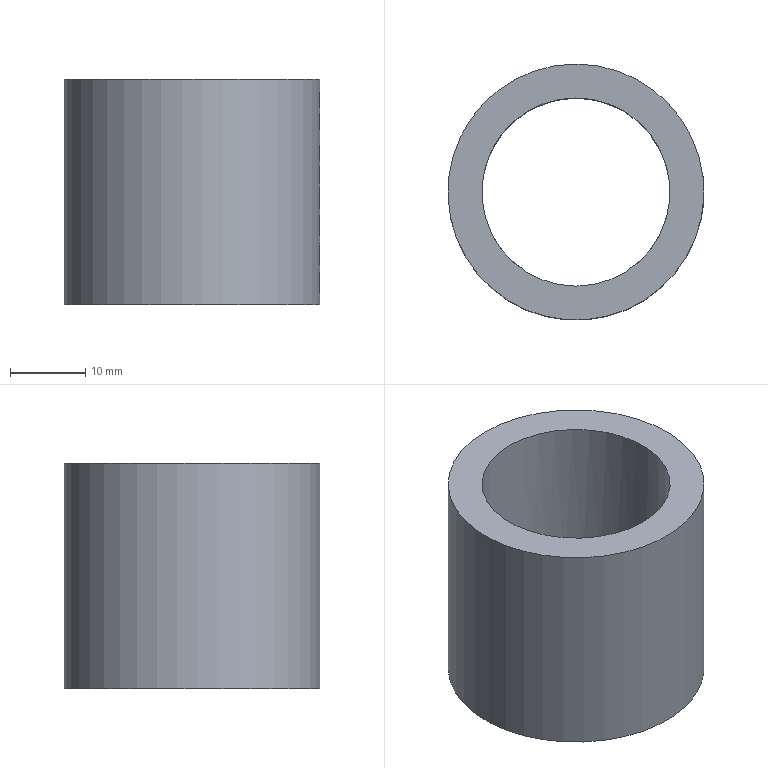Part | NX | features 25 2 | 1 solid | 136 faces | box 34.001 x 34 x 30 mm | volume 12501 mm3 | plane 70 | cylinder 63 | torus 3 | commonest cylinder face diameters 33.8 x9 25 x4 2.297 x2 34 x2 1.087 x1 1.125 x1